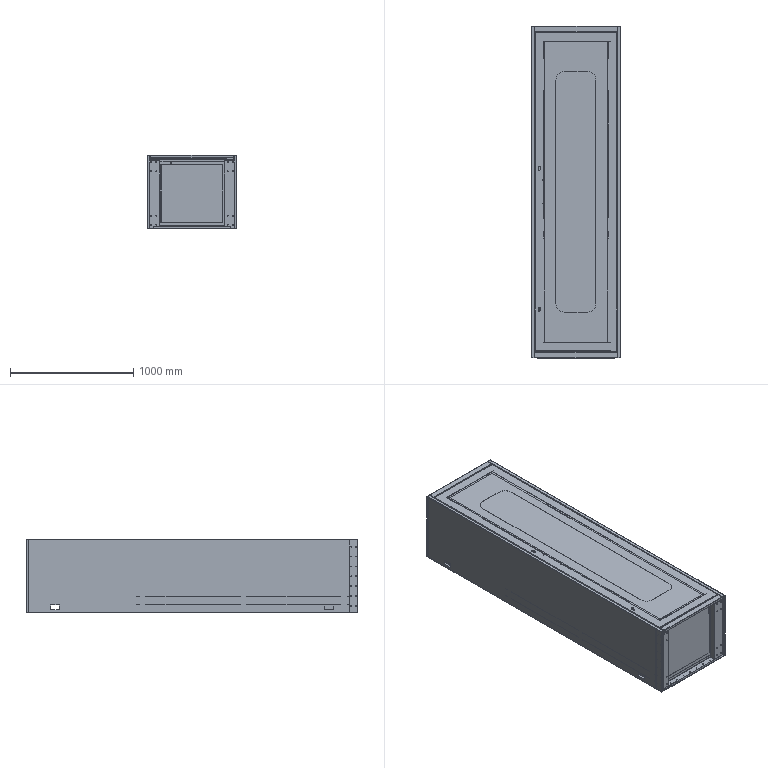Part | SolidWorks | features ReferencePattern 9, MirrorCompFeat 5, LocalLPattern 2, AEMSimFeature 1 | 108 solids | 6192 faces | volume 30600871 mm3 | plane 3716 | cylinder 2408 | spline 68 | commonest cylinder face diameters 4 x601 2 x567 6 x310 1.686 x252 3 x233 6.5 x84